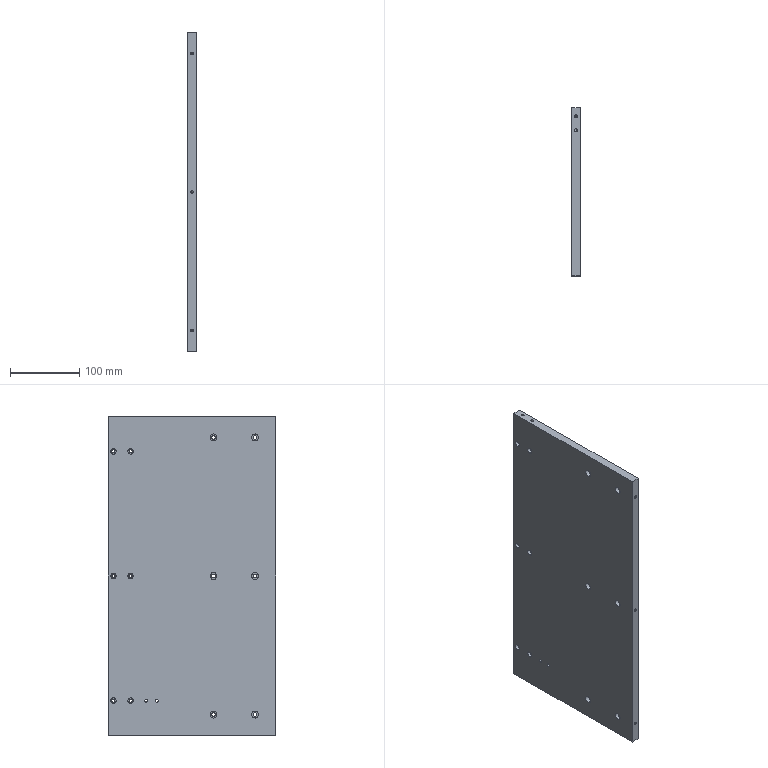Part | SolidWorks | features HoleWzd 5, Extrusion 1, MirrorPattern 1 | 1 solid | 98 faces | box 12 x 242 x 460 mm | volume 1328431 mm3 | cylinder 66 | plane 18 | cone 14 | commonest cylinder face diameters 4.2 x18 4.5 x12 5.5 x12 8 x12 10 x12